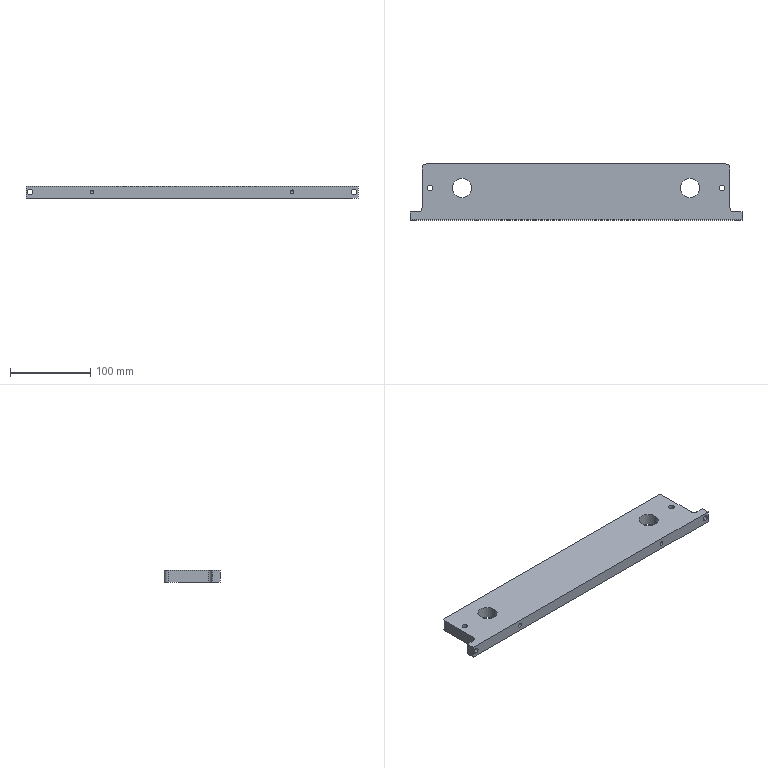Part | SolidWorks | features Fillet 2, HoleWzd 2, ICE 2, Extrusion 1 | 1 solid | 34 faces | box 415 x 70 x 15 mm | volume 392754 mm3 | cylinder 20 | plane 10 | cone 4 | commonest cylinder face diameters 6.8 x8 5 x4 10 x4 24 x4
STEP:
#1=CARTESIAN_POINT('',(-125.,-20.,10.));
#2=VERTEX_POINT('',#1);
#3=CARTESIAN_POINT('',(-125.,-20.,5.));
#4=VERTEX_POINT('',#3);
#5=CARTESIAN_POINT('',(-125.,-20.,7.5));
#6=DIRECTION('',(0.,-1.,0.));
#7=DIRECTION('',(0.,0.,-1.));
#8=AXIS2_PLACEMENT_3D('',#5,#6,#7);
#9=CIRCLE('',#8,2.5);
#10=EDGE_CURVE('',#2,#4,#9,.T.);
#11=ORIENTED_EDGE('',*,*,#10,.F.);
#12=CARTESIAN_POINT('',(-125.,-35.,10.));
#13=VERTEX_POINT('',#12);
#14=CARTESIAN_POINT('',(-125.,-35.,10.));
#15=DIRECTION('',(0.,-1.,0.));
#16=VECTOR('',#15,1000.);
#17=LINE('',#14,#16);
#18=EDGE_CURVE('',#2,#13,#17,.T.);
#19=ORIENTED_EDGE('',*,*,#18,.T.);
#20=CARTESIAN_POINT('',(-125.,-35.,5.));
#21=VERTEX_POINT('',#20);
#22=CARTESIAN_POINT('',(-125.,-35.,7.5));
#23=DIRECTION('',(0.,-1.,0.));
#24=DIRECTION('',(0.,0.,-1.));
#25=AXIS2_PLACEMENT_3D('',#22,#23,#24);
#26=CIRCLE('',#25,2.5);
#27=EDGE_CURVE('',#13,#21,#26,.T.);
#28=ORIENTED_EDGE('',*,*,#27,.T.);
#29=CARTESIAN_POINT('',(-125.,-35.,5.));
#30=DIRECTION('',(0.,-1.,0.));
#31=VECTOR('',#30,1000.);
#32=LINE('',#29,#31);
#33=EDGE_CURVE('',#4,#21,#32,.T.);
#34=ORIENTED_EDGE('',*,*,#33,.F.);
#35=EDGE_LOOP('',(#11,#19,#28,#34));
#36=FACE_OUTER_BOUND('',#35,.T.);
#37=CARTESIAN_POINT('',(-125.,-35.,7.5));
#38=DIRECTION('',(0.,-1.,0.));
#39=DIRECTION('',(0.,0.,-1.));
#40=AXIS2_PLACEMENT_3D('',#37,#38,#39);
#41=CYLINDRICAL_SURFACE('',#40,2.5);
#42=ADVANCED_FACE('',(#36),#41,.F.);
#43=CARTESIAN_POINT('',(-125.,-18.498,7.5));
#44=VERTEX_POINT('',#43);
#45=CARTESIAN_POINT('',(-125.,-20.,5.));
#46=DIRECTION('',(0.,-0.515,-0.8572));
#47=VECTOR('',#46,1000.);
#48=LINE('',#45,#47);
#49=EDGE_CURVE('',#44,#4,#48,.T.);
#50=ORIENTED_EDGE('',*,*,#49,.F.);
#51=CARTESIAN_POINT('',(-125.,-20.,10.));
#52=DIRECTION('',(0.,-0.515,0.8572));
#53=VECTOR('',#52,1000.);
#54=LINE('',#51,#53);
#55=EDGE_CURVE('',#44,#2,#54,.T.);
#56=ORIENTED_EDGE('',*,*,#55,.T.);
#57=ORIENTED_EDGE('',*,*,#10,.T.);
#58=EDGE_LOOP('',(#50,#56,#57));
#59=FACE_OUTER_BOUND('',#58,.T.);
#60=CARTESIAN_POINT('',(-125.,-20.,7.5));
#61=DIRECTION('',(0.,-1.,0.));
#62=DIRECTION('',(0.,0.,-1.));
#63=AXIS2_PLACEMENT_3D('',#60,#61,#62);
#64=CONICAL_SURFACE('',#63,2.5,1.03);
#65=ADVANCED_FACE('',(#59),#64,.F.);
#66=CARTESIAN_POINT('',(125.,-20.,10.));
#67=VERTEX_POINT('',#66);
#68=CARTESIAN_POINT('',(125.,-20.,5.));
#69=VERTEX_POINT('',#68);
#70=CARTESIAN_POINT('',(125.,-20.,7.5));
#71=DIRECTION('',(0.,-1.,0.));
#72=DIRECTION('',(0.,0.,-1.));
#73=AXIS2_PLACEMENT_3D('',#70,#71,#72);
#74=CIRCLE('',#73,2.5);
#75=EDGE_CURVE('',#67,#69,#74,.T.);
#76=ORIENTED_EDGE('',*,*,#75,.F.);
#77=CARTESIAN_POINT('',(125.,-35.,10.));
#78=VERTEX_POINT('',#77);
#79=CARTESIAN_POINT('',(125.,-35.,10.));
#80=DIRECTION('',(0.,-1.,0.));
#81=VECTOR('',#80,1000.);
#82=LINE('',#79,#81);
#83=EDGE_CURVE('',#67,#78,#82,.T.);
#84=ORIENTED_EDGE('',*,*,#83,.T.);
#85=CARTESIAN_POINT('',(125.,-35.,5.));
#86=VERTEX_POINT('',#85);
#87=CARTESIAN_POINT('',(125.,-35.,7.5));
#88=DIRECTION('',(0.,-1.,0.));
#89=DIRECTION('',(0.,0.,-1.));
#90=AXIS2_PLACEMENT_3D('',#87,#88,#89);
#91=CIRCLE('',#90,2.5);
#92=EDGE_CURVE('',#78,#86,#91,.T.);
#93=ORIENTED_EDGE('',*,*,#92,.T.);
#94=CARTESIAN_POINT('',(125.,-35.,5.));
#95=DIRECTION('',(0.,-1.,0.));
#96=VECTOR('',#95,1000.);
#97=LINE('',#94,#96);
#98=EDGE_CURVE('',#69,#86,#97,.T.);
#99=ORIENTED_EDGE('',*,*,#98,.F.);
#100=EDGE_LOOP('',(#76,#84,#93,#99));
#101=FACE_OUTER_BOUND('',#100,.T.);
#102=CARTESIAN_POINT('',(125.,-35.,7.5));
#103=DIRECTION('',(0.,-1.,0.));
#104=DIRECTION('',(0.,0.,-1.));
#105=AXIS2_PLACEMENT_3D('',#102,#103,#104);
#106=CYLINDRICAL_SURFACE('',#105,2.5);
#107=ADVANCED_FACE('',(#101),#106,.F.);
#108=CARTESIAN_POINT('',(125.,-18.498,7.5));
#109=VERTEX_POINT('',#108);
#110=CARTESIAN_POINT('',(125.,-20.,5.));
#111=DIRECTION('',(0.,-0.515,-0.8572));
#112=VECTOR('',#111,1000.);
#113=LINE('',#110,#112);
#114=EDGE_CURVE('',#109,#69,#113,.T.);
#115=ORIENTED_EDGE('',*,*,#114,.F.);
#116=CARTESIAN_POINT('',(125.,-20.,10.));
#117=DIRECTION('',(0.,-0.515,0.8572));
#118=VECTOR('',#117,1000.);
#119=LINE('',#116,#118);
#120=EDGE_CURVE('',#109,#67,#119,.T.);
#121=ORIENTED_EDGE('',*,*,#120,.T.);
#122=ORIENTED_EDGE('',*,*,#75,.T.);
#123=EDGE_LOOP('',(#115,#121,#122));
#124=FACE_OUTER_BOUND('',#123,.T.);
#125=CARTESIAN_POINT('',(125.,-20.,7.5));
#126=DIRECTION('',(0.,-1.,0.));
#127=DIRECTION('',(0.,0.,-1.));
#128=AXIS2_PLACEMENT_3D('',#125,#126,#127);
#129=CONICAL_SURFACE('',#128,2.5,1.03);
#130=ADVANCED_FACE('',(#124),#129,.F.);
#131=CARTESIAN_POINT('',(202.5,-25.,10.9));
#132=VERTEX_POINT('',#131);
#133=CARTESIAN_POINT('',(202.5,-25.,4.1));
#134=VERTEX_POINT('',#133);
#135=CARTESIAN_POINT('',(202.5,-25.,7.5));
#136=DIRECTION('',(0.,-1.,0.));
#137=DIRECTION('',(0.,0.,-1.));
#138=AXIS2_PLACEMENT_3D('',#135,#136,#137);
#139=CIRCLE('',#138,3.4);
#140=EDGE_CURVE('',#132,#134,#139,.T.);
#141=ORIENTED_EDGE('',*,*,#140,.F.);
#142=CARTESIAN_POINT('',(202.5,-35.,10.9));
#143=VERTEX_POINT('',#142);
#144=CARTESIAN_POINT('',(202.5,-35.,10.9));
#145=DIRECTION('',(0.,-1.,0.));
#146=VECTOR('',#145,1000.);
#147=LINE('',#144,#146);
#148=EDGE_CURVE('',#132,#143,#147,.T.);
#149=ORIENTED_EDGE('',*,*,#148,.T.);
#150=CARTESIAN_POINT('',(202.5,-35.,4.1));
#151=VERTEX_POINT('',#150);
#152=CARTESIAN_POINT('',(202.5,-35.,7.5));
#153=DIRECTION('',(0.,-1.,0.));
#154=DIRECTION('',(0.,0.,-1.));
#155=AXIS2_PLACEMENT_3D('',#152,#153,#154);
#156=CIRCLE('',#155,3.4);
#157=EDGE_CURVE('',#143,#151,#156,.T.);
#158=ORIENTED_EDGE('',*,*,#157,.T.);
#159=CARTESIAN_POINT('',(202.5,-35.,4.1));
#160=DIRECTION('',(0.,-1.,0.));
#161=VECTOR('',#160,1000.);
#162=LINE('',#159,#161);
#163=EDGE_CURVE('',#134,#151,#162,.T.);
#164=ORIENTED_EDGE('',*,*,#163,.F.);
#165=EDGE_LOOP('',(#141,#149,#158,#164));
#166=FACE_OUTER_BOUND('',#165,.T.);
#167=CARTESIAN_POINT('',(202.5,-35.,7.5));
#168=DIRECTION('',(0.,-1.,0.));
#169=DIRECTION('',(0.,0.,-1.));
#170=AXIS2_PLACEMENT_3D('',#167,#168,#169);
#171=CYLINDRICAL_SURFACE('',#170,3.4);
#172=ADVANCED_FACE('',(#166),#171,.F.);
#173=CARTESIAN_POINT('',(-202.5,-25.,10.9));
#174=VERTEX_POINT('',#173);
#175=CARTESIAN_POINT('',(-202.5,-25.,4.1));
#176=VERTEX_POINT('',#175);
#177=CARTESIAN_POINT('',(-202.5,-25.,7.5));
#178=DIRECTION('',(0.,-1.,0.));
#179=DIRECTION('',(0.,0.,-1.));
#180=AXIS2_PLACEMENT_3D('',#177,#178,#179);
#181=CIRCLE('',#180,3.4);
#182=EDGE_CURVE('',#174,#176,#181,.T.);
#183=ORIENTED_EDGE('',*,*,#182,.F.);
#184=CARTESIAN_POINT('',(-202.5,-35.,10.9));
#185=VERTEX_POINT('',#184);
#186=CARTESIAN_POINT('',(-202.5,-35.,10.9));
#187=DIRECTION('',(0.,-1.,0.));
#188=VECTOR('',#187,1000.);
#189=LINE('',#186,#188);
#190=EDGE_CURVE('',#174,#185,#189,.T.);
#191=ORIENTED_EDGE('',*,*,#190,.T.);
#192=CARTESIAN_POINT('',(-202.5,-35.,4.1));
#193=VERTEX_POINT('',#192);
#194=CARTESIAN_POINT('',(-202.5,-35.,7.5));
#195=DIRECTION('',(0.,-1.,0.));
#196=DIRECTION('',(0.,0.,-1.));
#197=AXIS2_PLACEMENT_3D('',#194,#195,#196);
#198=CIRCLE('',#197,3.4);
#199=EDGE_CURVE('',#185,#193,#198,.T.);
#200=ORIENTED_EDGE('',*,*,#199,.T.);
#201=CARTESIAN_POINT('',(-202.5,-35.,4.1));
#202=DIRECTION('',(0.,-1.,0.));
#203=VECTOR('',#202,1000.);
#204=LINE('',#201,#203);
#205=EDGE_CURVE('',#176,#193,#204,.T.);
#206=ORIENTED_EDGE('',*,*,#205,.F.);
#207=EDGE_LOOP('',(#183,#191,#200,#206));
#208=FACE_OUTER_BOUND('',#207,.T.);
#209=CARTESIAN_POINT('',(-202.5,-35.,7.5));
#210=DIRECTION('',(0.,-1.,0.));
#211=DIRECTION('',(0.,0.,-1.));
#212=AXIS2_PLACEMENT_3D('',#209,#210,#211);
#213=CYLINDRICAL_SURFACE('',#212,3.4);
#214=ADVANCED_FACE('',(#208),#213,.F.);
#215=CARTESIAN_POINT('',(179.1,5.,0.));
#216=VERTEX_POINT('',#215);
#217=CARTESIAN_POINT('',(185.9,5.,0.));
#218=VERTEX_POINT('',#217);
#219=CARTESIAN_POINT('',(182.5,5.,0.));
#220=DIRECTION('',(0.,0.,1.));
#221=DIRECTION('',(1.,0.,0.));
#222=AXIS2_PLACEMENT_3D('',#219,#220,#221);
#223=CIRCLE('',#222,3.4);
#224=EDGE_CURVE('',#216,#218,#223,.T.);
#225=ORIENTED_EDGE('',*,*,#224,.F.);
#226=CARTESIAN_POINT('',(179.1,5.,15.));
#227=VERTEX_POINT('',#226);
#228=CARTESIAN_POINT('',(179.1,5.,0.));
#229=DIRECTION('',(0.,0.,1.));
#230=VECTOR('',#229,1000.);
#231=LINE('',#228,#230);
#232=EDGE_CURVE('',#216,#227,#231,.T.);
#233=ORIENTED_EDGE('',*,*,#232,.T.);
#234=CARTESIAN_POINT('',(185.9,5.,15.));
#235=VERTEX_POINT('',#234);
#236=CARTESIAN_POINT('',(182.5,5.,15.));
#237=DIRECTION('',(0.,0.,1.));
#238=DIRECTION('',(1.,0.,0.));
#239=AXIS2_PLACEMENT_3D('',#236,#237,#238);
#240=CIRCLE('',#239,3.4);
#241=EDGE_CURVE('',#227,#235,#240,.T.);
#242=ORIENTED_EDGE('',*,*,#241,.T.);
#243=CARTESIAN_POINT('',(185.9,5.,0.));
#244=DIRECTION('',(0.,0.,1.));
#245=VECTOR('',#244,1000.);
#246=LINE('',#243,#245);
#247=EDGE_CURVE('',#218,#235,#246,.T.);
#248=ORIENTED_EDGE('',*,*,#247,.F.);
#249=EDGE_LOOP('',(#225,#233,#242,#248));
#250=FACE_OUTER_BOUND('',#249,.T.);
#251=CARTESIAN_POINT('',(182.5,5.,0.));
#252=DIRECTION('',(0.,0.,1.));
#253=DIRECTION('',(1.,0.,0.));
#254=AXIS2_PLACEMENT_3D('',#251,#252,#253);
#255=CYLINDRICAL_SURFACE('',#254,3.4);
#256=ADVANCED_FACE('',(#250),#255,.F.);
#257=CARTESIAN_POINT('',(-154.5,5.,0.));
#258=VERTEX_POINT('',#257);
#259=CARTESIAN_POINT('',(-130.5,5.,0.));
#260=VERTEX_POINT('',#259);
#261=CARTESIAN_POINT('',(-142.5,5.,0.));
#262=DIRECTION('',(0.,0.,1.));
#263=DIRECTION('',(1.,0.,0.));
#264=AXIS2_PLACEMENT_3D('',#261,#262,#263);
#265=CIRCLE('',#264,12.);
#266=EDGE_CURVE('',#258,#260,#265,.T.);
#267=ORIENTED_EDGE('',*,*,#266,.F.);
#268=CARTESIAN_POINT('',(-154.5,5.,15.));
#269=VERTEX_POINT('',#268);
#270=CARTESIAN_POINT('',(-154.5,5.,0.));
#271=DIRECTION('',(0.,0.,1.));
#272=VECTOR('',#271,1000.);
#273=LINE('',#270,#272);
#274=EDGE_CURVE('',#258,#269,#273,.T.);
#275=ORIENTED_EDGE('',*,*,#274,.T.);
#276=CARTESIAN_POINT('',(-130.5,5.,15.));
#277=VERTEX_POINT('',#276);
#278=CARTESIAN_POINT('',(-142.5,5.,15.));
#279=DIRECTION('',(0.,0.,1.));
#280=DIRECTION('',(1.,0.,0.));
#281=AXIS2_PLACEMENT_3D('',#278,#279,#280);
#282=CIRCLE('',#281,12.);
#283=EDGE_CURVE('',#269,#277,#282,.T.);
#284=ORIENTED_EDGE('',*,*,#283,.T.);
#285=CARTESIAN_POINT('',(-130.5,5.,0.));
#286=DIRECTION('',(0.,0.,1.));
#287=VECTOR('',#286,1000.);
#288=LINE('',#285,#287);
#289=EDGE_CURVE('',#260,#277,#288,.T.);
#290=ORIENTED_EDGE('',*,*,#289,.F.);
#291=EDGE_LOOP('',(#267,#275,#284,#290));
#292=FACE_OUTER_BOUND('',#291,.T.);
#293=CARTESIAN_POINT('',(-142.5,5.,0.));
#294=DIRECTION('',(0.,0.,1.));
#295=DIRECTION('',(1.,0.,0.));
#296=AXIS2_PLACEMENT_3D('',#293,#294,#295);
#297=CYLINDRICAL_SURFACE('',#296,12.);
#298=ADVANCED_FACE('',(#292),#297,.F.);
#299=CARTESIAN_POINT('',(-185.9,5.,0.));
#300=VERTEX_POINT('',#299);
#301=CARTESIAN_POINT('',(-179.1,5.,0.));
#302=VERTEX_POINT('',#301);
#303=CARTESIAN_POINT('',(-182.5,5.,0.));
#304=DIRECTION('',(0.,0.,1.));
#305=DIRECTION('',(1.,0.,0.));
#306=AXIS2_PLACEMENT_3D('',#303,#304,#305);
#307=CIRCLE('',#306,3.4);
#308=EDGE_CURVE('',#300,#302,#307,.T.);
#309=ORIENTED_EDGE('',*,*,#308,.F.);
#310=CARTESIAN_POINT('',(-185.9,5.,15.));
#311=VERTEX_POINT('',#310);
#312=CARTESIAN_POINT('',(-185.9,5.,0.));
#313=DIRECTION('',(0.,0.,1.));
#314=VECTOR('',#313,1000.);
#315=LINE('',#312,#314);
#316=EDGE_CURVE('',#300,#311,#315,.T.);
#317=ORIENTED_EDGE('',*,*,#316,.T.);
#318=CARTESIAN_POINT('',(-179.1,5.,15.));
#319=VERTEX_POINT('',#318);
#320=CARTESIAN_POINT('',(-182.5,5.,15.));
#321=DIRECTION('',(0.,0.,1.));
#322=DIRECTION('',(1.,0.,0.));
#323=AXIS2_PLACEMENT_3D('',#320,#321,#322);
#324=CIRCLE('',#323,3.4);
#325=EDGE_CURVE('',#311,#319,#324,.T.);
#326=ORIENTED_EDGE('',*,*,#325,.T.);
#327=CARTESIAN_POINT('',(-179.1,5.,0.));
#328=DIRECTION('',(0.,0.,1.));
#329=VECTOR('',#328,1000.);
#330=LINE('',#327,#329);
#331=EDGE_CURVE('',#302,#319,#330,.T.);
#332=ORIENTED_EDGE('',*,*,#331,.F.);
#333=EDGE_LOOP('',(#309,#317,#326,#332));
#334=FACE_OUTER_BOUND('',#333,.T.);
#335=CARTESIAN_POINT('',(-182.5,5.,0.));
#336=DIRECTION('',(0.,0.,1.));
#337=DIRECTION('',(1.,0.,0.));
#338=AXIS2_PLACEMENT_3D('',#335,#336,#337);
#339=CYLINDRICAL_SURFACE('',#338,3.4);
#340=ADVANCED_FACE('',(#334),#339,.F.);
#341=CARTESIAN_POINT('',(130.5,5.,0.));
#342=VERTEX_POINT('',#341);
#343=CARTESIAN_POINT('',(154.5,5.,0.));
#344=VERTEX_POINT('',#343);
#345=CARTESIAN_POINT('',(142.5,5.,0.));
#346=DIRECTION('',(0.,0.,1.));
#347=DIRECTION('',(1.,0.,0.));
#348=AXIS2_PLACEMENT_3D('',#345,#346,#347);
#349=CIRCLE('',#348,12.);
#350=EDGE_CURVE('',#342,#344,#349,.T.);
#351=ORIENTED_EDGE('',*,*,#350,.F.);
#352=CARTESIAN_POINT('',(130.5,5.,15.));
#353=VERTEX_POINT('',#352);
#354=CARTESIAN_POINT('',(130.5,5.,0.));
#355=DIRECTION('',(0.,0.,1.));
#356=VECTOR('',#355,1000.);
#357=LINE('',#354,#356);
#358=EDGE_CURVE('',#342,#353,#357,.T.);
#359=ORIENTED_EDGE('',*,*,#358,.T.);
#360=CARTESIAN_POINT('',(154.5,5.,15.));
#361=VERTEX_POINT('',#360);
#362=CARTESIAN_POINT('',(142.5,5.,15.));
#363=DIRECTION('',(0.,0.,1.));
#364=DIRECTION('',(1.,0.,0.));
#365=AXIS2_PLACEMENT_3D('',#362,#363,#364);
#366=CIRCLE('',#365,12.);
#367=EDGE_CURVE('',#353,#361,#366,.T.);
#368=ORIENTED_EDGE('',*,*,#367,.T.);
#369=CARTESIAN_POINT('',(154.5,5.,0.));
#370=DIRECTION('',(0.,0.,1.));
#371=VECTOR('',#370,1000.);
#372=LINE('',#369,#371);
#373=EDGE_CURVE('',#344,#361,#372,.T.);
#374=ORIENTED_EDGE('',*,*,#373,.F.);
#375=EDGE_LOOP('',(#351,#359,#368,#374));
#376=FACE_OUTER_BOUND('',#375,.T.);
#377=CARTESIAN_POINT('',(142.5,5.,0.));
#378=DIRECTION('',(0.,0.,1.));
#379=DIRECTION('',(1.,0.,0.));
#380=AXIS2_PLACEMENT_3D('',#377,#378,#379);
#381=CYLINDRICAL_SURFACE('',#380,12.);
#382=ADVANCED_FACE('',(#376),#381,.F.);
#383=CARTESIAN_POINT('',(-207.5,-25.,15.));
#384=VERTEX_POINT('',#383);
#385=CARTESIAN_POINT('',(-207.5,-35.,15.));
#386=VERTEX_POINT('',#385);
#387=CARTESIAN_POINT('',(-207.5,-35.,15.));
#388=DIRECTION('',(0.,-1.,0.));
#389=VECTOR('',#388,1000.);
#390=LINE('',#387,#389);
#391=EDGE_CURVE('',#384,#386,#390,.T.);
#392=ORIENTED_EDGE('',*,*,#391,.F.);
#393=CARTESIAN_POINT('',(-207.5,-25.,0.));
#394=VERTEX_POINT('',#393);
#395=CARTESIAN_POINT('',(-207.5,-25.,0.));
#396=DIRECTION('',(0.,0.,1.));
#397=VECTOR('',#396,1000.);
#398=LINE('',#395,#397);
#399=EDGE_CURVE('',#394,#384,#398,.T.);
#400=ORIENTED_EDGE('',*,*,#399,.F.);
#401=CARTESIAN_POINT('',(-207.5,-35.,0.));
#402=VERTEX_POINT('',#401);
#403=CARTESIAN_POINT('',(-207.5,-35.,0.));
#404=DIRECTION('',(0.,-1.,0.));
#405=VECTOR('',#404,1000.);
#406=LINE('',#403,#405);
#407=EDGE_CURVE('',#394,#402,#406,.T.);
#408=ORIENTED_EDGE('',*,*,#407,.T.);
#409=CARTESIAN_POINT('',(-207.5,-35.,15.));
#410=DIRECTION('',(0.,0.,-1.));
#411=VECTOR('',#410,1000.);
#412=LINE('',#409,#411);
#413=EDGE_CURVE('',#386,#402,#412,.T.);
#414=ORIENTED_EDGE('',*,*,#413,.F.);
#415=EDGE_LOOP('',(#392,#400,#408,#414));
#416=FACE_OUTER_BOUND('',#415,.T.);
#417=CARTESIAN_POINT('',(-207.5,-35.,15.));
#418=DIRECTION('',(1.,0.,0.));
#419=DIRECTION('',(0.,0.,-1.));
#420=AXIS2_PLACEMENT_3D('',#417,#418,#419);
#421=PLANE('',#420);
#422=ADVANCED_FACE('',(#416),#421,.F.);
#423=CARTESIAN_POINT('',(-125.,-35.,7.5));
#424=DIRECTION('',(0.,-1.,0.));
#425=DIRECTION('',(0.,0.,-1.));
#426=AXIS2_PLACEMENT_3D('',#423,#424,#425);
#427=CIRCLE('',#426,2.5);
#428=EDGE_CURVE('',#21,#13,#427,.T.);
#429=ORIENTED_EDGE('',*,*,#428,.F.);
#430=ORIENTED_EDGE('',*,*,#27,.F.);
#431=EDGE_LOOP('',(#429,#430));
#432=FACE_BOUND('',#431,.T.);
#433=CARTESIAN_POINT('',(125.,-35.,7.5));
#434=DIRECTION('',(0.,-1.,0.));
#435=DIRECTION('',(0.,0.,-1.));
#436=AXIS2_PLACEMENT_3D('',#433,#434,#435);
#437=CIRCLE('',#436,2.5);
#438=EDGE_CURVE('',#86,#78,#437,.T.);
#439=ORIENTED_EDGE('',*,*,#438,.F.);
#440=ORIENTED_EDGE('',*,*,#92,.F.);
#441=EDGE_LOOP('',(#439,#440));
#442=FACE_BOUND('',#441,.T.);
#443=CARTESIAN_POINT('',(202.5,-35.,7.5));
#444=DIRECTION('',(0.,-1.,0.));
#445=DIRECTION('',(0.,0.,-1.));
#446=AXIS2_PLACEMENT_3D('',#443,#444,#445);
#447=CIRCLE('',#446,3.4);
#448=EDGE_CURVE('',#151,#143,#447,.T.);
#449=ORIENTED_EDGE('',*,*,#448,.F.);
#450=ORIENTED_EDGE('',*,*,#157,.F.);
#451=EDGE_LOOP('',(#449,#450));
#452=FACE_BOUND('',#451,.T.);
#453=CARTESIAN_POINT('',(-202.5,-35.,7.5));
#454=DIRECTION('',(0.,-1.,0.));
#455=DIRECTION('',(0.,0.,-1.));
#456=AXIS2_PLACEMENT_3D('',#453,#454,#455);
#457=CIRCLE('',#456,3.4);
#458=EDGE_CURVE('',#193,#185,#457,.T.);
#459=ORIENTED_EDGE('',*,*,#458,.F.);
#460=ORIENTED_EDGE('',*,*,#199,.F.);
#461=EDGE_LOOP('',(#459,#460));
#462=FACE_BOUND('',#461,.T.);
#463=CARTESIAN_POINT('',(207.5,-35.,0.));
#464=VERTEX_POINT('',#463);
#465=CARTESIAN_POINT('',(207.5,-35.,0.));
#466=DIRECTION('',(1.,0.,0.));
#467=VECTOR('',#466,1000.);
#468=LINE('',#465,#467);
#469=EDGE_CURVE('',#402,#464,#468,.T.);
#470=ORIENTED_EDGE('',*,*,#469,.T.);
#471=CARTESIAN_POINT('',(207.5,-35.,15.));
#472=VERTEX_POINT('',#471);
#473=CARTESIAN_POINT('',(207.5,-35.,15.));
#474=DIRECTION('',(0.,0.,-1.));
#475=VECTOR('',#474,1000.);
#476=LINE('',#473,#475);
#477=EDGE_CURVE('',#472,#464,#476,.T.);
#478=ORIENTED_EDGE('',*,*,#477,.F.);
#479=CARTESIAN_POINT('',(207.5,-35.,15.));
#480=DIRECTION('',(1.,0.,0.));
#481=VECTOR('',#480,1000.);
#482=LINE('',#479,#481);
#483=EDGE_CURVE('',#386,#472,#482,.T.);
#484=ORIENTED_EDGE('',*,*,#483,.F.);
#485=ORIENTED_EDGE('',*,*,#413,.T.);
#486=EDGE_LOOP('',(#470,#478,#484,#485));
#487=FACE_OUTER_BOUND('',#486,.T.);
#488=CARTESIAN_POINT('',(207.5,-35.,15.));
#489=DIRECTION('',(0.,1.,0.));
#490=DIRECTION('',(-1.,0.,0.));
#491=AXIS2_PLACEMENT_3D('',#488,#489,#490);
#492=PLANE('',#491);
#493=ADVANCED_FACE('',(#432,#442,#452,#462,#487),#492,.F.);
#494=CARTESIAN_POINT('',(207.5,-25.,0.));
#495=VERTEX_POINT('',#494);
#496=CARTESIAN_POINT('',(207.5,-35.,0.));
#497=DIRECTION('',(0.,1.,0.));
#498=VECTOR('',#497,1000.);
#499=LINE('',#496,#498);
#500=EDGE_CURVE('',#464,#495,#499,.T.);
#501=ORIENTED_EDGE('',*,*,#500,.T.);
#502=CARTESIAN_POINT('',(207.5,-25.,15.));
#503=VERTEX_POINT('',#502);
#504=CARTESIAN_POINT('',(207.5,-25.,0.));
#505=DIRECTION('',(0.,0.,1.));
#506=VECTOR('',#505,1000.);
#507=LINE('',#504,#506);
#508=EDGE_CURVE('',#495,#503,#507,.T.);
#509=ORIENTED_EDGE('',*,*,#508,.T.);
#510=CARTESIAN_POINT('',(207.5,-35.,15.));
#511=DIRECTION('',(0.,1.,0.));
#512=VECTOR('',#511,1000.);
#513=LINE('',#510,#512);
#514=EDGE_CURVE('',#472,#503,#513,.T.);
#515=ORIENTED_EDGE('',*,*,#514,.F.);
#516=ORIENTED_EDGE('',*,*,#477,.T.);
#517=EDGE_LOOP('',(#501,#509,#515,#516));
#518=FACE_OUTER_BOUND('',#517,.T.);
#519=CARTESIAN_POINT('',(207.5,-35.,15.));
#520=DIRECTION('',(-1.,0.,0.));
#521=DIRECTION('',(0.,0.,1.));
#522=AXIS2_PLACEMENT_3D('',#519,#520,#521);
#523=PLANE('',#522);
#524=ADVANCED_FACE('',(#518),#523,.F.);
#525=CARTESIAN_POINT('',(187.5,35.,0.));
#526=VERTEX_POINT('',#525);
#527=CARTESIAN_POINT('',(-187.5,35.,0.));
#528=VERTEX_POINT('',#527);
#529=CARTESIAN_POINT('',(207.5,35.,0.));
#530=DIRECTION('',(-1.,0.,0.));
#531=VECTOR('',#530,1000.);
#532=LINE('',#529,#531);
#533=EDGE_CURVE('',#526,#528,#532,.T.);
#534=ORIENTED_EDGE('',*,*,#533,.T.);
#535=CARTESIAN_POINT('',(-187.5,35.,15.));
#536=VERTEX_POINT('',#535);
#537=CARTESIAN_POINT('',(-187.5,35.,15.));
#538=DIRECTION('',(0.,0.,1.));
#539=VECTOR('',#538,1000.);
#540=LINE('',#537,#539);
#541=EDGE_CURVE('',#528,#536,#540,.T.);
#542=ORIENTED_EDGE('',*,*,#541,.T.);
#543=CARTESIAN_POINT('',(187.5,35.,15.));
#544=VERTEX_POINT('',#543);
#545=CARTESIAN_POINT('',(207.5,35.,15.));
#546=DIRECTION('',(-1.,0.,0.));
#547=VECTOR('',#546,1000.);
#548=LINE('',#545,#547);
#549=EDGE_CURVE('',#544,#536,#548,.T.);
#550=ORIENTED_EDGE('',*,*,#549,.F.);
#551=CARTESIAN_POINT('',(187.5,35.,15.));
#552=DIRECTION('',(0.,0.,-1.));
#553=VECTOR('',#552,1000.);
#554=LINE('',#551,#553);
#555=EDGE_CURVE('',#544,#526,#554,.T.);
#556=ORIENTED_EDGE('',*,*,#555,.T.);
#557=EDGE_LOOP('',(#534,#542,#550,#556));
#558=FACE_OUTER_BOUND('',#557,.T.);
#559=CARTESIAN_POINT('',(207.5,35.,15.));
#560=DIRECTION('',(0.,-1.,0.));
#561=DIRECTION('',(1.,0.,0.));
#562=AXIS2_PLACEMENT_3D('',#559,#560,#561);
#563=PLANE('',#562);
#564=ADVANCED_FACE('',(#558),#563,.F.);
#565=ORIENTED_EDGE('',*,*,#549,.T.);
#566=CARTESIAN_POINT('',(-192.5,30.,15.));
#567=VERTEX_POINT('',#566);
#568=CARTESIAN_POINT('',(-187.5,30.,15.));
#569=DIRECTION('',(0.,0.,1.));
#570=DIRECTION('',(1.,0.,0.));
#571=AXIS2_PLACEMENT_3D('',#568,#569,#570);
#572=CIRCLE('',#571,5.);
#573=EDGE_CURVE('',#536,#567,#572,.T.);
#574=ORIENTED_EDGE('',*,*,#573,.T.);
#575=CARTESIAN_POINT('',(-192.5,-20.,15.));
#576=VERTEX_POINT('',#575);
#577=CARTESIAN_POINT('',(-192.5,35.,15.));
#578=DIRECTION('',(0.,1.,0.));
#579=VECTOR('',#578,1000.);
#580=LINE('',#577,#579);
#581=EDGE_CURVE('',#576,#567,#580,.T.);
#582=ORIENTED_EDGE('',*,*,#581,.F.);
#583=CARTESIAN_POINT('',(-197.5,-25.,15.));
#584=VERTEX_POINT('',#583);
#585=CARTESIAN_POINT('',(-197.5,-20.,15.));
#586=DIRECTION('',(0.,0.,-1.));
#587=DIRECTION('',(1.,0.,0.));
#588=AXIS2_PLACEMENT_3D('',#585,#586,#587);
#589=CIRCLE('',#588,5.);
#590=EDGE_CURVE('',#576,#584,#589,.T.);
#591=ORIENTED_EDGE('',*,*,#590,.T.);
#592=CARTESIAN_POINT('',(-207.5,-25.,15.));
#593=DIRECTION('',(1.,0.,0.));
#594=VECTOR('',#593,1000.);
#595=LINE('',#592,#594);
#596=EDGE_CURVE('',#384,#584,#595,.T.);
#597=ORIENTED_EDGE('',*,*,#596,.F.);
#598=ORIENTED_EDGE('',*,*,#391,.T.);
#599=ORIENTED_EDGE('',*,*,#483,.T.);
#600=ORIENTED_EDGE('',*,*,#514,.T.);
#601=CARTESIAN_POINT('',(197.5,-25.,15.));
#602=VERTEX_POINT('',#601);
#603=CARTESIAN_POINT('',(207.5,-25.,15.));
#604=DIRECTION('',(1.,0.,0.));
#605=VECTOR('',#604,1000.);
#606=LINE('',#603,#605);
#607=EDGE_CURVE('',#602,#503,#606,.T.);
#608=ORIENTED_EDGE('',*,*,#607,.F.);
#609=CARTESIAN_POINT('',(192.5,-20.,15.));
#610=VERTEX_POINT('',#609);
#611=CARTESIAN_POINT('',(197.5,-20.,15.));
#612=DIRECTION('',(0.,0.,-1.));
#613=DIRECTION('',(1.,0.,0.));
#614=AXIS2_PLACEMENT_3D('',#611,#612,#613);
#615=CIRCLE('',#614,5.);
#616=EDGE_CURVE('',#602,#610,#615,.T.);
#617=ORIENTED_EDGE('',*,*,#616,.T.);
#618=CARTESIAN_POINT('',(192.5,30.,15.));
#619=VERTEX_POINT('',#618);
#620=CARTESIAN_POINT('',(192.5,35.,15.));
#621=DIRECTION('',(0.,-1.,0.));
#622=VECTOR('',#621,1000.);
#623=LINE('',#620,#622);
#624=EDGE_CURVE('',#619,#610,#623,.T.);
#625=ORIENTED_EDGE('',*,*,#624,.F.);
#626=CARTESIAN_POINT('',(187.5,30.,15.));
#627=DIRECTION('',(0.,0.,1.));
#628=DIRECTION('',(1.,0.,0.));
#629=AXIS2_PLACEMENT_3D('',#626,#627,#628);
#630=CIRCLE('',#629,5.);
#631=EDGE_CURVE('',#619,#544,#630,.T.);
#632=ORIENTED_EDGE('',*,*,#631,.T.);
#633=EDGE_LOOP('',(#565,#574,#582,#591,#597,#598,#599,#600,#608,#617,#625,#632));
#634=FACE_OUTER_BOUND('',#633,.T.);
#635=CARTESIAN_POINT('',(182.5,5.,15.));
#636=DIRECTION('',(0.,0.,1.));
#637=DIRECTION('',(1.,0.,0.));
#638=AXIS2_PLACEMENT_3D('',#635,#636,#637);
#639=CIRCLE('',#638,3.4);
#640=EDGE_CURVE('',#235,#227,#639,.T.);
#641=ORIENTED_EDGE('',*,*,#640,.F.);
#642=ORIENTED_EDGE('',*,*,#241,.F.);
#643=EDGE_LOOP('',(#641,#642));
#644=FACE_BOUND('',#643,.T.);
#645=CARTESIAN_POINT('',(-142.5,5.,15.));
#646=DIRECTION('',(0.,0.,1.));
#647=DIRECTION('',(1.,0.,0.));
#648=AXIS2_PLACEMENT_3D('',#645,#646,#647);
#649=CIRCLE('',#648,12.);
#650=EDGE_CURVE('',#277,#269,#649,.T.);
#651=ORIENTED_EDGE('',*,*,#650,.F.);
#652=ORIENTED_EDGE('',*,*,#283,.F.);
#653=EDGE_LOOP('',(#651,#652));
#654=FACE_BOUND('',#653,.T.);
#655=CARTESIAN_POINT('',(-182.5,5.,15.));
#656=DIRECTION('',(0.,0.,1.));
#657=DIRECTION('',(1.,0.,0.));
#658=AXIS2_PLACEMENT_3D('',#655,#656,#657);
#659=CIRCLE('',#658,3.4);
#660=EDGE_CURVE('',#319,#311,#659,.T.);
#661=ORIENTED_EDGE('',*,*,#660,.F.);
#662=ORIENTED_EDGE('',*,*,#325,.F.);
#663=EDGE_LOOP('',(#661,#662));
#664=FACE_BOUND('',#663,.T.);
#665=CARTESIAN_POINT('',(142.5,5.,15.));
#666=DIRECTION('',(0.,0.,1.));
#667=DIRECTION('',(1.,0.,0.));
#668=AXIS2_PLACEMENT_3D('',#665,#666,#667);
#669=CIRCLE('',#668,12.);
#670=EDGE_CURVE('',#361,#353,#669,.T.);
#671=ORIENTED_EDGE('',*,*,#670,.F.);
#672=ORIENTED_EDGE('',*,*,#367,.F.);
#673=EDGE_LOOP('',(#671,#672));
#674=FACE_BOUND('',#673,.T.);
#675=CARTESIAN_POINT('',(0.,0.,15.));
#676=DIRECTION('',(0.,0.,1.));
#677=DIRECTION('',(1.,0.,0.));
#678=AXIS2_PLACEMENT_3D('',#675,#676,#677);
#679=PLANE('',#678);
#680=ADVANCED_FACE('',(#634,#644,#654,#664,#674),#679,.T.);
#681=CARTESIAN_POINT('',(182.5,5.,0.));
#682=DIRECTION('',(0.,0.,1.));
#683=DIRECTION('',(1.,0.,0.));
#684=AXIS2_PLACEMENT_3D('',#681,#682,#683);
#685=CIRCLE('',#684,3.4);
#686=EDGE_CURVE('',#218,#216,#685,.T.);
#687=ORIENTED_EDGE('',*,*,#686,.T.);
#688=ORIENTED_EDGE('',*,*,#224,.T.);
#689=EDGE_LOOP('',(#687,#688));
#690=FACE_BOUND('',#689,.T.);
#691=CARTESIAN_POINT('',(-142.5,5.,0.));
#692=DIRECTION('',(0.,0.,1.));
#693=DIRECTION('',(1.,0.,0.));
#694=AXIS2_PLACEMENT_3D('',#691,#692,#693);
#695=CIRCLE('',#694,12.);
#696=EDGE_CURVE('',#260,#258,#695,.T.);
#697=ORIENTED_EDGE('',*,*,#696,.T.);
#698=ORIENTED_EDGE('',*,*,#266,.T.);
#699=EDGE_LOOP('',(#697,#698));
#700=FACE_BOUND('',#699,.T.);
#701=CARTESIAN_POINT('',(-182.5,5.,0.));
#702=DIRECTION('',(0.,0.,1.));
#703=DIRECTION('',(1.,0.,0.));
#704=AXIS2_PLACEMENT_3D('',#701,#702,#703);
#705=CIRCLE('',#704,3.4);
#706=EDGE_CURVE('',#302,#300,#705,.T.);
#707=ORIENTED_EDGE('',*,*,#706,.T.);
#708=ORIENTED_EDGE('',*,*,#308,.T.);
#709=EDGE_LOOP('',(#707,#708));
#710=FACE_BOUND('',#709,.T.);
#711=CARTESIAN_POINT('',(142.5,5.,0.));
#712=DIRECTION('',(0.,0.,1.));
#713=DIRECTION('',(1.,0.,0.));
#714=AXIS2_PLACEMENT_3D('',#711,#712,#713);
#715=CIRCLE('',#714,12.);
#716=EDGE_CURVE('',#344,#342,#715,.T.);
#717=ORIENTED_EDGE('',*,*,#716,.T.);
#718=ORIENTED_EDGE('',*,*,#350,.T.);
#719=EDGE_LOOP('',(#717,#718));
#720=FACE_BOUND('',#719,.T.);
#721=CARTESIAN_POINT('',(-192.5,-20.,0.));
#722=VERTEX_POINT('',#721);
#723=CARTESIAN_POINT('',(-192.5,30.,0.));
#724=VERTEX_POINT('',#723);
#725=CARTESIAN_POINT('',(-192.5,35.,0.));
#726=DIRECTION('',(0.,1.,0.));
#727=VECTOR('',#726,1000.);
#728=LINE('',#725,#727);
#729=EDGE_CURVE('',#722,#724,#728,.T.);
#730=ORIENTED_EDGE('',*,*,#729,.T.);
#731=CARTESIAN_POINT('',(-187.5,30.,0.));
#732=DIRECTION('',(0.,0.,-1.));
#733=DIRECTION('',(1.,0.,0.));
#734=AXIS2_PLACEMENT_3D('',#731,#732,#733);
#735=CIRCLE('',#734,5.);
#736=EDGE_CURVE('',#724,#528,#735,.T.);
#737=ORIENTED_EDGE('',*,*,#736,.T.);
#738=ORIENTED_EDGE('',*,*,#533,.F.);
#739=CARTESIAN_POINT('',(192.5,30.,0.));
#740=VERTEX_POINT('',#739);
#741=CARTESIAN_POINT('',(187.5,30.,0.));
#742=DIRECTION('',(0.,0.,-1.));
#743=DIRECTION('',(1.,0.,0.));
#744=AXIS2_PLACEMENT_3D('',#741,#742,#743);
#745=CIRCLE('',#744,5.);
#746=EDGE_CURVE('',#526,#740,#745,.T.);
#747=ORIENTED_EDGE('',*,*,#746,.T.);
#748=CARTESIAN_POINT('',(192.5,-20.,0.));
#749=VERTEX_POINT('',#748);
#750=CARTESIAN_POINT('',(192.5,35.,0.));
#751=DIRECTION('',(0.,-1.,0.));
#752=VECTOR('',#751,1000.);
#753=LINE('',#750,#752);
#754=EDGE_CURVE('',#740,#749,#753,.T.);
#755=ORIENTED_EDGE('',*,*,#754,.T.);
#756=CARTESIAN_POINT('',(197.5,-25.,0.));
#757=VERTEX_POINT('',#756);
#758=CARTESIAN_POINT('',(197.5,-20.,0.));
#759=DIRECTION('',(0.,0.,1.));
#760=DIRECTION('',(1.,0.,0.));
#761=AXIS2_PLACEMENT_3D('',#758,#759,#760);
#762=CIRCLE('',#761,5.);
#763=EDGE_CURVE('',#749,#757,#762,.T.);
#764=ORIENTED_EDGE('',*,*,#763,.T.);
#765=CARTESIAN_POINT('',(207.5,-25.,0.));
#766=DIRECTION('',(1.,0.,0.));
#767=VECTOR('',#766,1000.);
#768=LINE('',#765,#767);
#769=EDGE_CURVE('',#757,#495,#768,.T.);
#770=ORIENTED_EDGE('',*,*,#769,.T.);
#771=ORIENTED_EDGE('',*,*,#500,.F.);
#772=ORIENTED_EDGE('',*,*,#469,.F.);
#773=ORIENTED_EDGE('',*,*,#407,.F.);
#774=CARTESIAN_POINT('',(-197.5,-25.,0.));
#775=VERTEX_POINT('',#774);
#776=CARTESIAN_POINT('',(-207.5,-25.,0.));
#777=DIRECTION('',(1.,0.,0.));
#778=VECTOR('',#777,1000.);
#779=LINE('',#776,#778);
#780=EDGE_CURVE('',#394,#775,#779,.T.);
#781=ORIENTED_EDGE('',*,*,#780,.T.);
#782=CARTESIAN_POINT('',(-197.5,-20.,0.));
#783=DIRECTION('',(0.,0.,1.));
#784=DIRECTION('',(1.,0.,0.));
#785=AXIS2_PLACEMENT_3D('',#782,#783,#784);
#786=CIRCLE('',#785,5.);
#787=EDGE_CURVE('',#775,#722,#786,.T.);
#788=ORIENTED_EDGE('',*,*,#787,.T.);
#789=EDGE_LOOP('',(#730,#737,#738,#747,#755,#764,#770,#771,#772,#773,#781,#788));
#790=FACE_OUTER_BOUND('',#789,.T.);
#791=CARTESIAN_POINT('',(0.,0.,0.));
#792=DIRECTION('',(0.,0.,1.));
#793=DIRECTION('',(1.,0.,0.));
#794=AXIS2_PLACEMENT_3D('',#791,#792,#793);
#795=PLANE('',#794);
#796=ADVANCED_FACE('',(#690,#700,#710,#720,#790),#795,.F.);
#797=ORIENTED_EDGE('',*,*,#358,.F.);
#798=ORIENTED_EDGE('',*,*,#716,.F.);
#799=ORIENTED_EDGE('',*,*,#373,.T.);
#800=ORIENTED_EDGE('',*,*,#670,.T.);
#801=EDGE_LOOP('',(#797,#798,#799,#800));
#802=FACE_OUTER_BOUND('',#801,.T.);
#803=CARTESIAN_POINT('',(142.5,5.,0.));
#804=DIRECTION('',(0.,0.,1.));
#805=DIRECTION('',(1.,0.,0.));
#806=AXIS2_PLACEMENT_3D('',#803,#804,#805);
#807=CYLINDRICAL_SURFACE('',#806,12.);
#808=ADVANCED_FACE('',(#802),#807,.F.);
#809=ORIENTED_EDGE('',*,*,#316,.F.);
#810=ORIENTED_EDGE('',*,*,#706,.F.);
#811=ORIENTED_EDGE('',*,*,#331,.T.);
#812=ORIENTED_EDGE('',*,*,#660,.T.);
#813=EDGE_LOOP('',(#809,#810,#811,#812));
#814=FACE_OUTER_BOUND('',#813,.T.);
#815=CARTESIAN_POINT('',(-182.5,5.,0.));
#816=DIRECTION('',(0.,0.,1.));
#817=DIRECTION('',(1.,0.,0.));
#818=AXIS2_PLACEMENT_3D('',#815,#816,#817);
#819=CYLINDRICAL_SURFACE('',#818,3.4);
#820=ADVANCED_FACE('',(#814),#819,.F.);
#821=ORIENTED_EDGE('',*,*,#274,.F.);
#822=ORIENTED_EDGE('',*,*,#696,.F.);
#823=ORIENTED_EDGE('',*,*,#289,.T.);
#824=ORIENTED_EDGE('',*,*,#650,.T.);
#825=EDGE_LOOP('',(#821,#822,#823,#824));
#826=FACE_OUTER_BOUND('',#825,.T.);
#827=CARTESIAN_POINT('',(-142.5,5.,0.));
#828=DIRECTION('',(0.,0.,1.));
#829=DIRECTION('',(1.,0.,0.));
#830=AXIS2_PLACEMENT_3D('',#827,#828,#829);
#831=CYLINDRICAL_SURFACE('',#830,12.);
#832=ADVANCED_FACE('',(#826),#831,.F.);
#833=ORIENTED_EDGE('',*,*,#232,.F.);
#834=ORIENTED_EDGE('',*,*,#686,.F.);
#835=ORIENTED_EDGE('',*,*,#247,.T.);
#836=ORIENTED_EDGE('',*,*,#640,.T.);
#837=EDGE_LOOP('',(#833,#834,#835,#836));
#838=FACE_OUTER_BOUND('',#837,.T.);
#839=CARTESIAN_POINT('',(182.5,5.,0.));
#840=DIRECTION('',(0.,0.,1.));
#841=DIRECTION('',(1.,0.,0.));
#842=AXIS2_PLACEMENT_3D('',#839,#840,#841);
#843=CYLINDRICAL_SURFACE('',#842,3.4);
#844=ADVANCED_FACE('',(#838),#843,.F.);
#845=CARTESIAN_POINT('',(202.5,-25.,7.5));
#846=DIRECTION('',(0.,-1.,0.));
#847=DIRECTION('',(0.,0.,-1.));
#848=AXIS2_PLACEMENT_3D('',#845,#846,#847);
#849=CIRCLE('',#848,3.4);
#850=EDGE_CURVE('',#134,#132,#849,.T.);
#851=ORIENTED_EDGE('',*,*,#850,.T.);
#852=ORIENTED_EDGE('',*,*,#140,.T.);
#853=EDGE_LOOP('',(#851,#852));
#854=FACE_BOUND('',#853,.T.);
#855=ORIENTED_EDGE('',*,*,#769,.F.);
#856=CARTESIAN_POINT('',(197.5,-25.,15.));
#857=DIRECTION('',(0.,0.,1.));
#858=VECTOR('',#857,1000.);
#859=LINE('',#856,#858);
#860=EDGE_CURVE('',#757,#602,#859,.T.);
#861=ORIENTED_EDGE('',*,*,#860,.T.);
#862=ORIENTED_EDGE('',*,*,#607,.T.);
#863=ORIENTED_EDGE('',*,*,#508,.F.);
#864=EDGE_LOOP('',(#855,#861,#862,#863));
#865=FACE_OUTER_BOUND('',#864,.T.);
#866=CARTESIAN_POINT('',(207.5,-25.,0.));
#867=DIRECTION('',(0.,-1.,0.));
#868=DIRECTION('',(0.,0.,-1.));
#869=AXIS2_PLACEMENT_3D('',#866,#867,#868);
#870=PLANE('',#869);
#871=ADVANCED_FACE('',(#854,#865),#870,.F.);
#872=ORIENTED_EDGE('',*,*,#754,.F.);
#873=CARTESIAN_POINT('',(192.5,30.,0.));
#874=DIRECTION('',(0.,0.,1.));
#875=VECTOR('',#874,1000.);
#876=LINE('',#873,#875);
#877=EDGE_CURVE('',#740,#619,#876,.T.);
#878=ORIENTED_EDGE('',*,*,#877,.T.);
#879=ORIENTED_EDGE('',*,*,#624,.T.);
#880=CARTESIAN_POINT('',(192.5,-20.,0.));
#881=DIRECTION('',(0.,0.,-1.));
#882=VECTOR('',#881,1000.);
#883=LINE('',#880,#882);
#884=EDGE_CURVE('',#610,#749,#883,.T.);
#885=ORIENTED_EDGE('',*,*,#884,.T.);
#886=EDGE_LOOP('',(#872,#878,#879,#885));
#887=FACE_OUTER_BOUND('',#886,.T.);
#888=CARTESIAN_POINT('',(192.5,35.,0.));
#889=DIRECTION('',(-1.,0.,0.));
#890=DIRECTION('',(0.,0.,1.));
#891=AXIS2_PLACEMENT_3D('',#888,#889,#890);
#892=PLANE('',#891);
#893=ADVANCED_FACE('',(#887),#892,.F.);
#894=ORIENTED_EDGE('',*,*,#581,.T.);
#895=CARTESIAN_POINT('',(-192.5,30.,0.));
#896=DIRECTION('',(0.,0.,-1.));
#897=VECTOR('',#896,1000.);
#898=LINE('',#895,#897);
#899=EDGE_CURVE('',#567,#724,#898,.T.);
#900=ORIENTED_EDGE('',*,*,#899,.T.);
#901=ORIENTED_EDGE('',*,*,#729,.F.);
#902=CARTESIAN_POINT('',(-192.5,-20.,15.));
#903=DIRECTION('',(0.,0.,1.));
#904=VECTOR('',#903,1000.);
#905=LINE('',#902,#904);
#906=EDGE_CURVE('',#722,#576,#905,.T.);
#907=ORIENTED_EDGE('',*,*,#906,.T.);
#908=EDGE_LOOP('',(#894,#900,#901,#907));
#909=FACE_OUTER_BOUND('',#908,.T.);
#910=CARTESIAN_POINT('',(-192.5,35.,0.));
#911=DIRECTION('',(1.,0.,0.));
#912=DIRECTION('',(0.,0.,-1.));
#913=AXIS2_PLACEMENT_3D('',#910,#911,#912);
#914=PLANE('',#913);
#915=ADVANCED_FACE('',(#909),#914,.F.);
#916=CARTESIAN_POINT('',(-202.5,-25.,7.5));
#917=DIRECTION('',(0.,-1.,0.));
#918=DIRECTION('',(0.,0.,-1.));
#919=AXIS2_PLACEMENT_3D('',#916,#917,#918);
#920=CIRCLE('',#919,3.4);
#921=EDGE_CURVE('',#176,#174,#920,.T.);
#922=ORIENTED_EDGE('',*,*,#921,.T.);
#923=ORIENTED_EDGE('',*,*,#182,.T.);
#924=EDGE_LOOP('',(#922,#923));
#925=FACE_BOUND('',#924,.T.);
#926=ORIENTED_EDGE('',*,*,#596,.T.);
#927=CARTESIAN_POINT('',(-197.5,-25.,0.));
#928=DIRECTION('',(0.,0.,-1.));
#929=VECTOR('',#928,1000.);
#930=LINE('',#927,#929);
#931=EDGE_CURVE('',#584,#775,#930,.T.);
#932=ORIENTED_EDGE('',*,*,#931,.T.);
#933=ORIENTED_EDGE('',*,*,#780,.F.);
#934=ORIENTED_EDGE('',*,*,#399,.T.);
#935=EDGE_LOOP('',(#926,#932,#933,#934));
#936=FACE_OUTER_BOUND('',#935,.T.);
#937=CARTESIAN_POINT('',(-207.5,-25.,0.));
#938=DIRECTION('',(0.,-1.,0.));
#939=DIRECTION('',(0.,0.,-1.));
#940=AXIS2_PLACEMENT_3D('',#937,#938,#939);
#941=PLANE('',#940);
#942=ADVANCED_FACE('',(#925,#936),#941,.F.);
#943=ORIENTED_EDGE('',*,*,#190,.F.);
#944=ORIENTED_EDGE('',*,*,#921,.F.);
#945=ORIENTED_EDGE('',*,*,#205,.T.);
#946=ORIENTED_EDGE('',*,*,#458,.T.);
#947=EDGE_LOOP('',(#943,#944,#945,#946));
#948=FACE_OUTER_BOUND('',#947,.T.);
#949=CARTESIAN_POINT('',(-202.5,-35.,7.5));
#950=DIRECTION('',(0.,-1.,0.));
#951=DIRECTION('',(0.,0.,-1.));
#952=AXIS2_PLACEMENT_3D('',#949,#950,#951);
#953=CYLINDRICAL_SURFACE('',#952,3.4);
#954=ADVANCED_FACE('',(#948),#953,.F.);
#955=ORIENTED_EDGE('',*,*,#148,.F.);
#956=ORIENTED_EDGE('',*,*,#850,.F.);
#957=ORIENTED_EDGE('',*,*,#163,.T.);
#958=ORIENTED_EDGE('',*,*,#448,.T.);
#959=EDGE_LOOP('',(#955,#956,#957,#958));
#960=FACE_OUTER_BOUND('',#959,.T.);
#961=CARTESIAN_POINT('',(202.5,-35.,7.5));
#962=DIRECTION('',(0.,-1.,0.));
#963=DIRECTION('',(0.,0.,-1.));
#964=AXIS2_PLACEMENT_3D('',#961,#962,#963);
#965=CYLINDRICAL_SURFACE('',#964,3.4);
#966=ADVANCED_FACE('',(#960),#965,.F.);
#967=ORIENTED_EDGE('',*,*,#763,.F.);
#968=ORIENTED_EDGE('',*,*,#884,.F.);
#969=ORIENTED_EDGE('',*,*,#616,.F.);
#970=ORIENTED_EDGE('',*,*,#860,.F.);
#971=EDGE_LOOP('',(#967,#968,#969,#970));
#972=FACE_OUTER_BOUND('',#971,.T.);
#973=CARTESIAN_POINT('',(197.5,-20.,0.));
#974=DIRECTION('',(0.,0.,-1.));
#975=DIRECTION('',(-1.,0.,0.));
#976=AXIS2_PLACEMENT_3D('',#973,#974,#975);
#977=CYLINDRICAL_SURFACE('',#976,5.);
#978=ADVANCED_FACE('',(#972),#977,.F.);
#979=ORIENTED_EDGE('',*,*,#787,.F.);
#980=ORIENTED_EDGE('',*,*,#931,.F.);
#981=ORIENTED_EDGE('',*,*,#590,.F.);
#982=ORIENTED_EDGE('',*,*,#906,.F.);
#983=EDGE_LOOP('',(#979,#980,#981,#982));
#984=FACE_OUTER_BOUND('',#983,.T.);
#985=CARTESIAN_POINT('',(-197.5,-20.,0.));
#986=DIRECTION('',(0.,0.,-1.));
#987=DIRECTION('',(-1.,0.,0.));
#988=AXIS2_PLACEMENT_3D('',#985,#986,#987);
#989=CYLINDRICAL_SURFACE('',#988,5.);
#990=ADVANCED_FACE('',(#984),#989,.F.);
#991=ORIENTED_EDGE('',*,*,#736,.F.);
#992=ORIENTED_EDGE('',*,*,#899,.F.);
#993=ORIENTED_EDGE('',*,*,#573,.F.);
#994=ORIENTED_EDGE('',*,*,#541,.F.);
#995=EDGE_LOOP('',(#991,#992,#993,#994));
#996=FACE_OUTER_BOUND('',#995,.T.);
#997=CARTESIAN_POINT('',(-187.5,30.,15.));
#998=DIRECTION('',(0.,0.,1.));
#999=DIRECTION('',(1.,0.,0.));
#1000=AXIS2_PLACEMENT_3D('',#997,#998,#999);
#1001=CYLINDRICAL_SURFACE('',#1000,5.);
#1002=ADVANCED_FACE('',(#996),#1001,.T.);
#1003=ORIENTED_EDGE('',*,*,#746,.F.);
#1004=ORIENTED_EDGE('',*,*,#555,.F.);
#1005=ORIENTED_EDGE('',*,*,#631,.F.);
#1006=ORIENTED_EDGE('',*,*,#877,.F.);
#1007=EDGE_LOOP('',(#1003,#1004,#1005,#1006));
#1008=FACE_OUTER_BOUND('',#1007,.T.);
#1009=CARTESIAN_POINT('',(187.5,30.,0.));
#1010=DIRECTION('',(0.,0.,1.));
#1011=DIRECTION('',(1.,0.,0.));
#1012=AXIS2_PLACEMENT_3D('',#1009,#1010,#1011);
#1013=CYLINDRICAL_SURFACE('',#1012,5.);
#1014=ADVANCED_FACE('',(#1008),#1013,.T.);
#1015=ORIENTED_EDGE('',*,*,#120,.F.);
#1016=ORIENTED_EDGE('',*,*,#114,.T.);
#1017=CARTESIAN_POINT('',(125.,-20.,7.5));
#1018=DIRECTION('',(0.,-1.,0.));
#1019=DIRECTION('',(0.,0.,-1.));
#1020=AXIS2_PLACEMENT_3D('',#1017,#1018,#1019);
#1021=CIRCLE('',#1020,2.5);
#1022=EDGE_CURVE('',#69,#67,#1021,.T.);
#1023=ORIENTED_EDGE('',*,*,#1022,.T.);
#1024=EDGE_LOOP('',(#1015,#1016,#1023));
#1025=FACE_OUTER_BOUND('',#1024,.T.);
#1026=CARTESIAN_POINT('',(125.,-20.,7.5));
#1027=DIRECTION('',(0.,-1.,0.));
#1028=DIRECTION('',(0.,0.,-1.));
#1029=AXIS2_PLACEMENT_3D('',#1026,#1027,#1028);
#1030=CONICAL_SURFACE('',#1029,2.5,1.03);
#1031=ADVANCED_FACE('',(#1025),#1030,.F.);
#1032=ORIENTED_EDGE('',*,*,#83,.F.);
#1033=ORIENTED_EDGE('',*,*,#1022,.F.);
#1034=ORIENTED_EDGE('',*,*,#98,.T.);
#1035=ORIENTED_EDGE('',*,*,#438,.T.);
#1036=EDGE_LOOP('',(#1032,#1033,#1034,#1035));
#1037=FACE_OUTER_BOUND('',#1036,.T.);
#1038=CARTESIAN_POINT('',(125.,-35.,7.5));
#1039=DIRECTION('',(0.,-1.,0.));
#1040=DIRECTION('',(0.,0.,-1.));
#1041=AXIS2_PLACEMENT_3D('',#1038,#1039,#1040);
#1042=CYLINDRICAL_SURFACE('',#1041,2.5);
#1043=ADVANCED_FACE('',(#1037),#1042,.F.);
#1044=ORIENTED_EDGE('',*,*,#55,.F.);
#1045=ORIENTED_EDGE('',*,*,#49,.T.);
#1046=CARTESIAN_POINT('',(-125.,-20.,7.5));
#1047=DIRECTION('',(0.,-1.,0.));
#1048=DIRECTION('',(0.,0.,-1.));
#1049=AXIS2_PLACEMENT_3D('',#1046,#1047,#1048);
#1050=CIRCLE('',#1049,2.5);
#1051=EDGE_CURVE('',#4,#2,#1050,.T.);
#1052=ORIENTED_EDGE('',*,*,#1051,.T.);
#1053=EDGE_LOOP('',(#1044,#1045,#1052));
#1054=FACE_OUTER_BOUND('',#1053,.T.);
#1055=CARTESIAN_POINT('',(-125.,-20.,7.5));
#1056=DIRECTION('',(0.,-1.,0.));
#1057=DIRECTION('',(0.,0.,-1.));
#1058=AXIS2_PLACEMENT_3D('',#1055,#1056,#1057);
#1059=CONICAL_SURFACE('',#1058,2.5,1.03);
#1060=ADVANCED_FACE('',(#1054),#1059,.F.);
#1061=ORIENTED_EDGE('',*,*,#18,.F.);
#1062=ORIENTED_EDGE('',*,*,#1051,.F.);
#1063=ORIENTED_EDGE('',*,*,#33,.T.);
#1064=ORIENTED_EDGE('',*,*,#428,.T.);
#1065=EDGE_LOOP('',(#1061,#1062,#1063,#1064));
#1066=FACE_OUTER_BOUND('',#1065,.T.);
#1067=CARTESIAN_POINT('',(-125.,-35.,7.5));
#1068=DIRECTION('',(0.,-1.,0.));
#1069=DIRECTION('',(0.,0.,-1.));
#1070=AXIS2_PLACEMENT_3D('',#1067,#1068,#1069);
#1071=CYLINDRICAL_SURFACE('',#1070,2.5);
#1072=ADVANCED_FACE('',(#1066),#1071,.F.);
#1073=CLOSED_SHELL('',(#42,#65,#107,#130,#172,#214,#256,#298,#340,#382,#422,#493,#524,#564,#680,#796,#808,#820,#832,#844,#871,#893,#915,#942,#954,#966,#978,#990,#1002,#1014,#1031,#1043,#1060,#1072));
#1074=MANIFOLD_SOLID_BREP('',#1073);
#1075=CARTESIAN_POINT('',(0.,0.,0.));
#1076=DIRECTION('',(0.,0.,1.));
#1077=DIRECTION('',(1.,0.,0.));
#1078=AXIS2_PLACEMENT_3D('',#1075,#1076,#1077);
#1079=(LENGTH_UNIT()NAMED_UNIT(*)SI_UNIT(.MILLI.,.METRE.));
#1080=UNCERTAINTY_MEASURE_WITH_UNIT(LENGTH_MEASURE(0.00001),#1079,'','');
#1081=(NAMED_UNIT(*)PLANE_ANGLE_UNIT()SI_UNIT($,.RADIAN.));
#1082=(NAMED_UNIT(*)SI_UNIT($,.STERADIAN.)SOLID_ANGLE_UNIT());
#1083=(GEOMETRIC_REPRESENTATION_CONTEXT(3)GLOBAL_UNCERTAINTY_ASSIGNED_CONTEXT((#1080))GLOBAL_UNIT_ASSIGNED_CONTEXT((#1079,#1081,#1082))REPRESENTATION_CONTEXT('',''));
#1084=ADVANCED_BREP_SHAPE_REPRESENTATION('',(#1074,#1078),#1083);